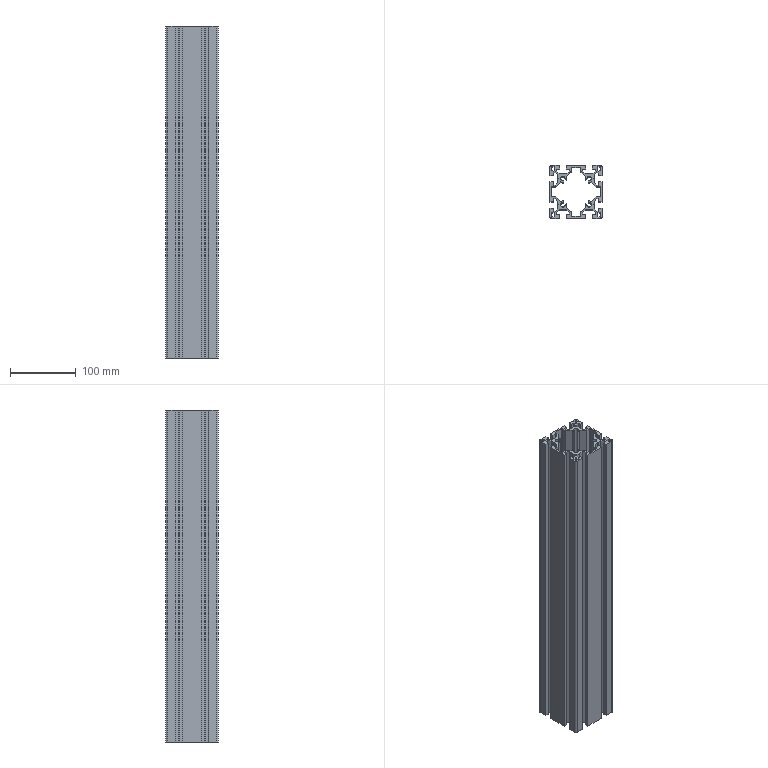Part | SolidWorks | features BaseBody 1 | 1 solid | 231 faces | box 80 x 80 x 505 mm | volume 860071 mm3 | plane 154 | cylinder 77 | commonest cylinder face diameters 2 x34 0.6 x17 6.8 x12 12 x10 6 x4